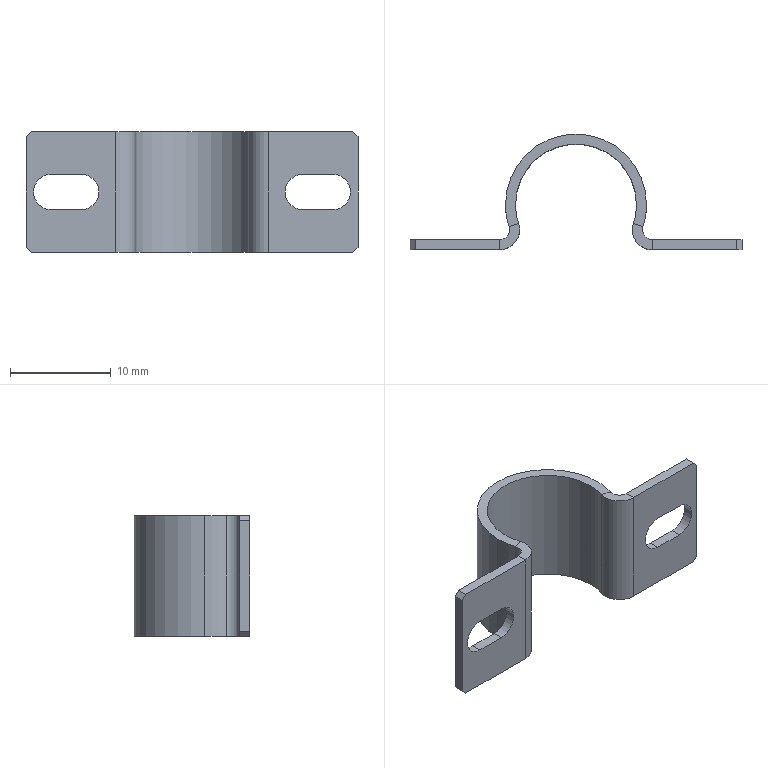Part | STEP file | 1 solid | 40 faces | box 33 x 11.5 x 12 mm | volume 535.489 mm3 | plane 24 | cylinder 16 | commonest cylinder face diameters 3.5 x4 2 x3 4 x3 12 x3 14 x3